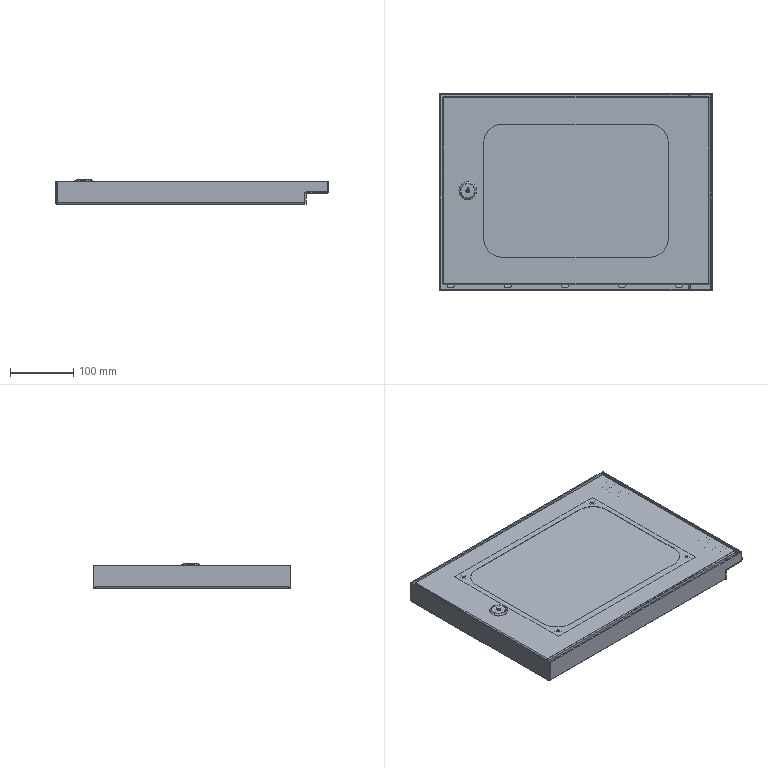Part | SolidWorks | 19 solids | 646 faces | box 430 x 310 x 39 mm | volume 586867 mm3 | plane 349 | cylinder 203 | cone 58 | spline 20 | torus 11 | sphere 5 | commonest cylinder face diameters 4 x31 5 x23 1 x20 3 x16 5.3 x16 6 x16